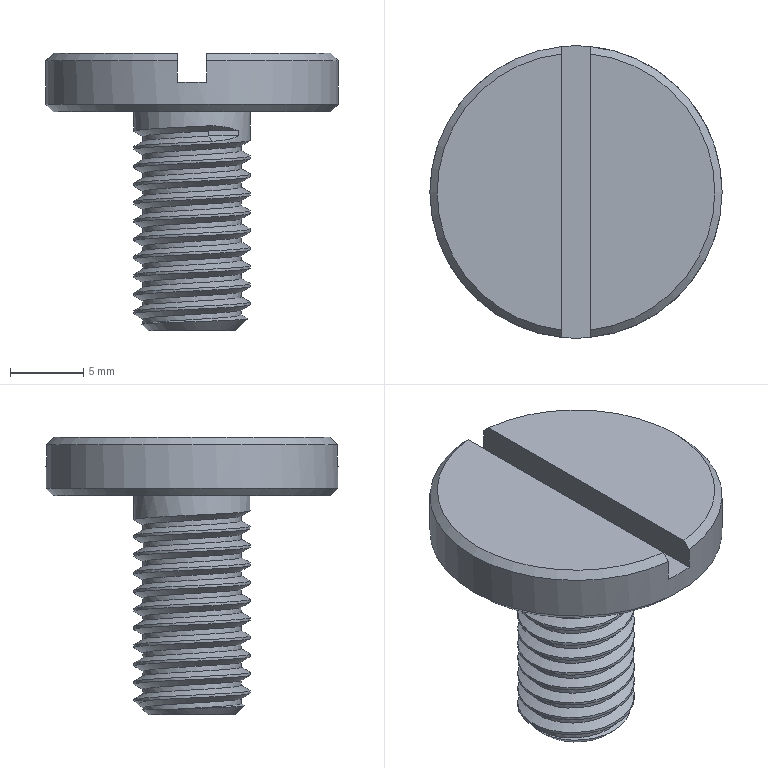Part | NX | features DATUM_CSYS 5, EXTRUDE 4, SKETCH 4, CHAMFER 2, THREADS 1 | 1 solid | 30 faces | box 20 x 20 x 19 mm | volume 1790 mm3 | cylinder 12 | plane 11 | cone 5 | spline 2 | commonest cylinder face diameters 8 x10 6.75 x1 20 x1